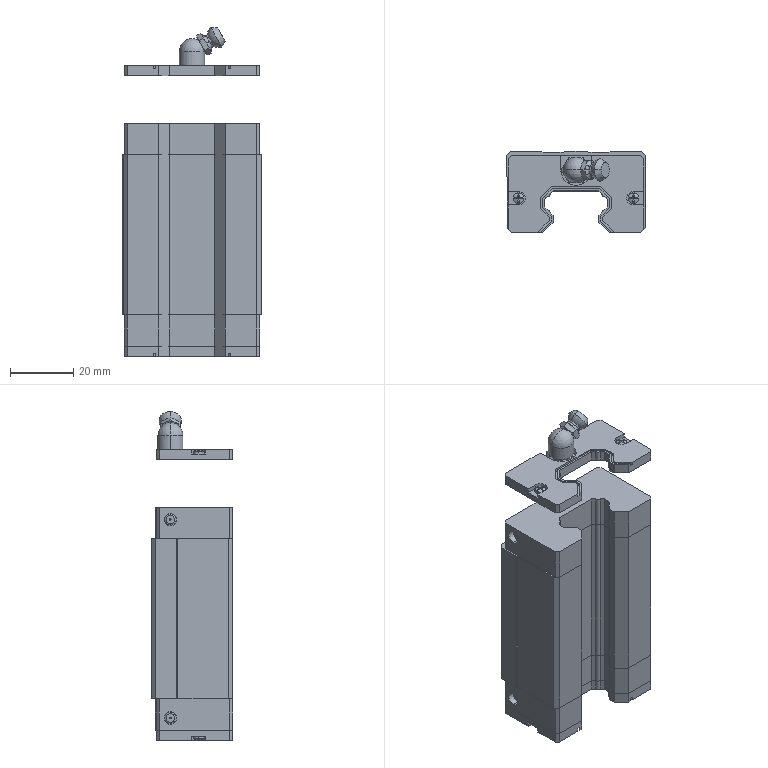Part | SolidWorks | features ICE 23, Extrusion 5, MirrorPattern 5, Fillet 4, MirrorSolid 4, Chamfer 3, Dome 2, Revolution 2, LibraryFeature 1, RevCut 1 | 6 solids | 836 faces | box 44 x 25.71 x 103.7 mm | volume 65250 mm3 | plane 565 | spline 119 | cylinder 86 | cone 31 | torus 25 | sphere 10 | commonest cylinder face diameters 1.817 x30 3.93 x12 0.531 x8 3.414 x8 4 x8 5 x8